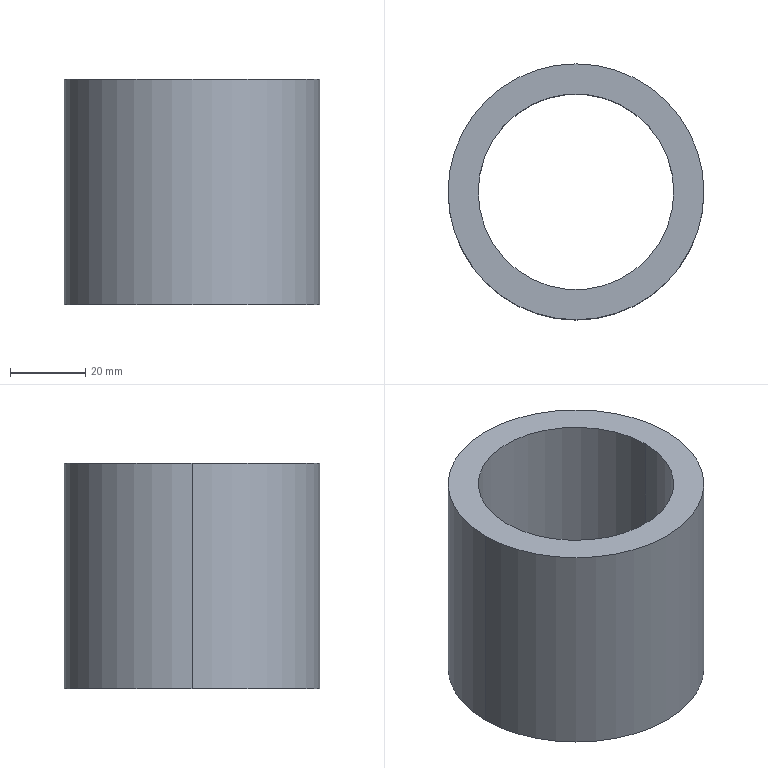Part | SolidWorks | features Extrusion 1, WeldmentFeature 1 | 1 solid | 6 faces | box 68 x 68 x 60 mm | volume 90478 mm3 | cylinder 4 | plane 2 | commonest cylinder face diameters 52 x2 68 x2
STEP:
#1=CARTESIAN_POINT('',(-26.,0.,60.));
#2=VERTEX_POINT('',#1);
#3=CARTESIAN_POINT('',(26.,0.,60.));
#4=VERTEX_POINT('',#3);
#5=CARTESIAN_POINT('',(0.,0.,60.));
#6=DIRECTION('',(0.,0.,1.));
#7=DIRECTION('',(1.,0.,0.));
#8=AXIS2_PLACEMENT_3D('',#5,#6,#7);
#9=CIRCLE('',#8,26.);
#10=EDGE_CURVE('',#2,#4,#9,.T.);
#11=ORIENTED_EDGE('',*,*,#10,.T.);
#12=CARTESIAN_POINT('',(26.,0.,0.));
#13=VERTEX_POINT('',#12);
#14=CARTESIAN_POINT('',(26.,0.,60.));
#15=DIRECTION('',(0.,0.,-1.));
#16=VECTOR('',#15,1000.);
#17=LINE('',#14,#16);
#18=EDGE_CURVE('',#4,#13,#17,.T.);
#19=ORIENTED_EDGE('',*,*,#18,.T.);
#20=CARTESIAN_POINT('',(-26.,0.,0.));
#21=VERTEX_POINT('',#20);
#22=CARTESIAN_POINT('',(0.,0.,0.));
#23=DIRECTION('',(0.,0.,1.));
#24=DIRECTION('',(1.,0.,0.));
#25=AXIS2_PLACEMENT_3D('',#22,#23,#24);
#26=CIRCLE('',#25,26.);
#27=EDGE_CURVE('',#21,#13,#26,.T.);
#28=ORIENTED_EDGE('',*,*,#27,.F.);
#29=CARTESIAN_POINT('',(-26.,0.,60.));
#30=DIRECTION('',(0.,0.,-1.));
#31=VECTOR('',#30,1000.);
#32=LINE('',#29,#31);
#33=EDGE_CURVE('',#2,#21,#32,.T.);
#34=ORIENTED_EDGE('',*,*,#33,.F.);
#35=EDGE_LOOP('',(#11,#19,#28,#34));
#36=FACE_OUTER_BOUND('',#35,.T.);
#37=CARTESIAN_POINT('',(0.,0.,60.));
#38=DIRECTION('',(0.,0.,-1.));
#39=DIRECTION('',(-1.,0.,0.));
#40=AXIS2_PLACEMENT_3D('',#37,#38,#39);
#41=CYLINDRICAL_SURFACE('',#40,26.);
#42=ADVANCED_FACE('',(#36),#41,.F.);
#43=CARTESIAN_POINT('',(34.,0.,60.));
#44=VERTEX_POINT('',#43);
#45=CARTESIAN_POINT('',(-34.,0.,60.));
#46=VERTEX_POINT('',#45);
#47=CARTESIAN_POINT('',(0.,0.,60.));
#48=DIRECTION('',(0.,0.,1.));
#49=DIRECTION('',(1.,0.,0.));
#50=AXIS2_PLACEMENT_3D('',#47,#48,#49);
#51=CIRCLE('',#50,34.);
#52=EDGE_CURVE('',#44,#46,#51,.T.);
#53=ORIENTED_EDGE('',*,*,#52,.F.);
#54=CARTESIAN_POINT('',(34.,0.,0.));
#55=VERTEX_POINT('',#54);
#56=CARTESIAN_POINT('',(34.,0.,60.));
#57=DIRECTION('',(0.,0.,-1.));
#58=VECTOR('',#57,1000.);
#59=LINE('',#56,#58);
#60=EDGE_CURVE('',#44,#55,#59,.T.);
#61=ORIENTED_EDGE('',*,*,#60,.T.);
#62=CARTESIAN_POINT('',(-34.,0.,0.));
#63=VERTEX_POINT('',#62);
#64=CARTESIAN_POINT('',(0.,0.,0.));
#65=DIRECTION('',(0.,0.,1.));
#66=DIRECTION('',(1.,0.,0.));
#67=AXIS2_PLACEMENT_3D('',#64,#65,#66);
#68=CIRCLE('',#67,34.);
#69=EDGE_CURVE('',#55,#63,#68,.T.);
#70=ORIENTED_EDGE('',*,*,#69,.T.);
#71=CARTESIAN_POINT('',(-34.,0.,60.));
#72=DIRECTION('',(0.,0.,-1.));
#73=VECTOR('',#72,1000.);
#74=LINE('',#71,#73);
#75=EDGE_CURVE('',#46,#63,#74,.T.);
#76=ORIENTED_EDGE('',*,*,#75,.F.);
#77=EDGE_LOOP('',(#53,#61,#70,#76));
#78=FACE_OUTER_BOUND('',#77,.T.);
#79=CARTESIAN_POINT('',(0.,0.,60.));
#80=DIRECTION('',(0.,0.,-1.));
#81=DIRECTION('',(-1.,0.,0.));
#82=AXIS2_PLACEMENT_3D('',#79,#80,#81);
#83=CYLINDRICAL_SURFACE('',#82,34.);
#84=ADVANCED_FACE('',(#78),#83,.T.);
#85=CARTESIAN_POINT('',(0.,0.,60.));
#86=DIRECTION('',(0.,0.,1.));
#87=DIRECTION('',(1.,0.,0.));
#88=AXIS2_PLACEMENT_3D('',#85,#86,#87);
#89=CIRCLE('',#88,34.);
#90=EDGE_CURVE('',#46,#44,#89,.T.);
#91=ORIENTED_EDGE('',*,*,#90,.T.);
#92=ORIENTED_EDGE('',*,*,#52,.T.);
#93=EDGE_LOOP('',(#91,#92));
#94=FACE_OUTER_BOUND('',#93,.T.);
#95=ORIENTED_EDGE('',*,*,#10,.F.);
#96=CARTESIAN_POINT('',(0.,0.,60.));
#97=DIRECTION('',(0.,0.,1.));
#98=DIRECTION('',(1.,0.,0.));
#99=AXIS2_PLACEMENT_3D('',#96,#97,#98);
#100=CIRCLE('',#99,26.);
#101=EDGE_CURVE('',#4,#2,#100,.T.);
#102=ORIENTED_EDGE('',*,*,#101,.F.);
#103=EDGE_LOOP('',(#95,#102));
#104=FACE_BOUND('',#103,.T.);
#105=CARTESIAN_POINT('',(0.,0.,60.));
#106=DIRECTION('',(0.,0.,1.));
#107=DIRECTION('',(1.,0.,0.));
#108=AXIS2_PLACEMENT_3D('',#105,#106,#107);
#109=PLANE('',#108);
#110=ADVANCED_FACE('',(#94,#104),#109,.T.);
#111=CARTESIAN_POINT('',(0.,0.,0.));
#112=DIRECTION('',(0.,0.,1.));
#113=DIRECTION('',(1.,0.,0.));
#114=AXIS2_PLACEMENT_3D('',#111,#112,#113);
#115=CIRCLE('',#114,34.);
#116=EDGE_CURVE('',#63,#55,#115,.T.);
#117=ORIENTED_EDGE('',*,*,#116,.F.);
#118=ORIENTED_EDGE('',*,*,#69,.F.);
#119=EDGE_LOOP('',(#117,#118));
#120=FACE_OUTER_BOUND('',#119,.T.);
#121=ORIENTED_EDGE('',*,*,#27,.T.);
#122=CARTESIAN_POINT('',(0.,0.,0.));
#123=DIRECTION('',(0.,0.,1.));
#124=DIRECTION('',(1.,0.,0.));
#125=AXIS2_PLACEMENT_3D('',#122,#123,#124);
#126=CIRCLE('',#125,26.);
#127=EDGE_CURVE('',#13,#21,#126,.T.);
#128=ORIENTED_EDGE('',*,*,#127,.T.);
#129=EDGE_LOOP('',(#121,#128));
#130=FACE_BOUND('',#129,.T.);
#131=CARTESIAN_POINT('',(0.,0.,0.));
#132=DIRECTION('',(0.,0.,1.));
#133=DIRECTION('',(1.,0.,0.));
#134=AXIS2_PLACEMENT_3D('',#131,#132,#133);
#135=PLANE('',#134);
#136=ADVANCED_FACE('',(#120,#130),#135,.F.);
#137=ORIENTED_EDGE('',*,*,#60,.F.);
#138=ORIENTED_EDGE('',*,*,#90,.F.);
#139=ORIENTED_EDGE('',*,*,#75,.T.);
#140=ORIENTED_EDGE('',*,*,#116,.T.);
#141=EDGE_LOOP('',(#137,#138,#139,#140));
#142=FACE_OUTER_BOUND('',#141,.T.);
#143=CARTESIAN_POINT('',(0.,0.,60.));
#144=DIRECTION('',(0.,0.,-1.));
#145=DIRECTION('',(-1.,0.,0.));
#146=AXIS2_PLACEMENT_3D('',#143,#144,#145);
#147=CYLINDRICAL_SURFACE('',#146,34.);
#148=ADVANCED_FACE('',(#142),#147,.T.);
#149=ORIENTED_EDGE('',*,*,#18,.F.);
#150=ORIENTED_EDGE('',*,*,#101,.T.);
#151=ORIENTED_EDGE('',*,*,#33,.T.);
#152=ORIENTED_EDGE('',*,*,#127,.F.);
#153=EDGE_LOOP('',(#149,#150,#151,#152));
#154=FACE_OUTER_BOUND('',#153,.T.);
#155=CARTESIAN_POINT('',(0.,0.,60.));
#156=DIRECTION('',(0.,0.,-1.));
#157=DIRECTION('',(-1.,0.,0.));
#158=AXIS2_PLACEMENT_3D('',#155,#156,#157);
#159=CYLINDRICAL_SURFACE('',#158,26.);
#160=ADVANCED_FACE('',(#154),#159,.F.);
#161=CLOSED_SHELL('',(#42,#84,#110,#136,#148,#160));
#162=MANIFOLD_SOLID_BREP('',#161);
#163=CARTESIAN_POINT('',(0.,0.,0.));
#164=DIRECTION('',(0.,0.,1.));
#165=DIRECTION('',(1.,0.,0.));
#166=AXIS2_PLACEMENT_3D('',#163,#164,#165);
#167=(LENGTH_UNIT()NAMED_UNIT(*)SI_UNIT(.MILLI.,.METRE.));
#168=UNCERTAINTY_MEASURE_WITH_UNIT(LENGTH_MEASURE(0.00001),#167,'','');
#169=(NAMED_UNIT(*)PLANE_ANGLE_UNIT()SI_UNIT($,.RADIAN.));
#170=(NAMED_UNIT(*)SI_UNIT($,.STERADIAN.)SOLID_ANGLE_UNIT());
#171=(GEOMETRIC_REPRESENTATION_CONTEXT(3)GLOBAL_UNCERTAINTY_ASSIGNED_CONTEXT((#168))GLOBAL_UNIT_ASSIGNED_CONTEXT((#167,#169,#170))REPRESENTATION_CONTEXT('',''));
#172=ADVANCED_BREP_SHAPE_REPRESENTATION('',(#162,#166),#171);